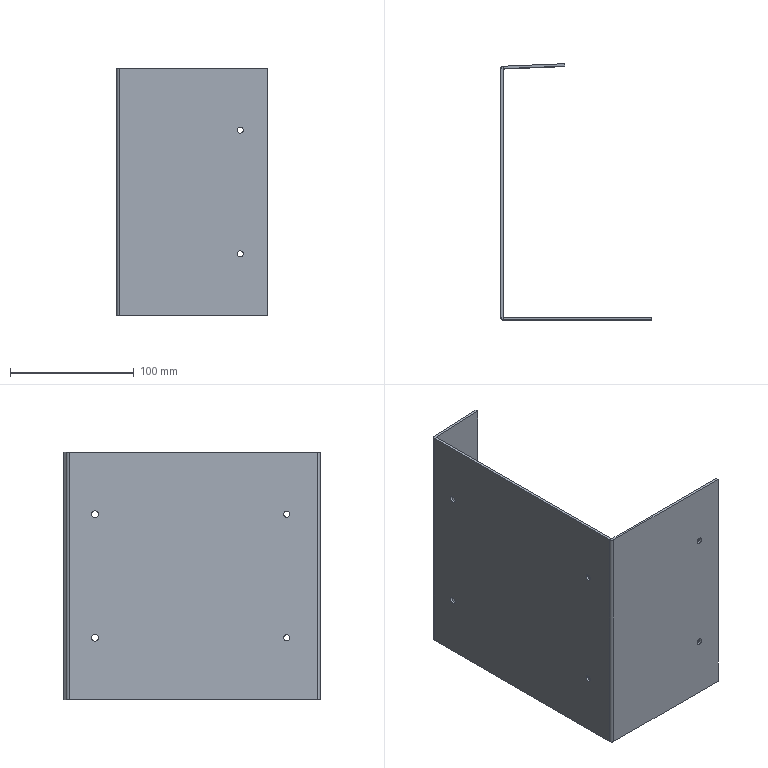Part | STEP file | TS-S23 | 1 solid | 34 faces | box 122 x 207.205 x 200 mm | volume 149406 mm3 | plane 18 | cylinder 16 | commonest cylinder face diameters 5 x8 5.4 x4 0.4 x2 4.4 x2